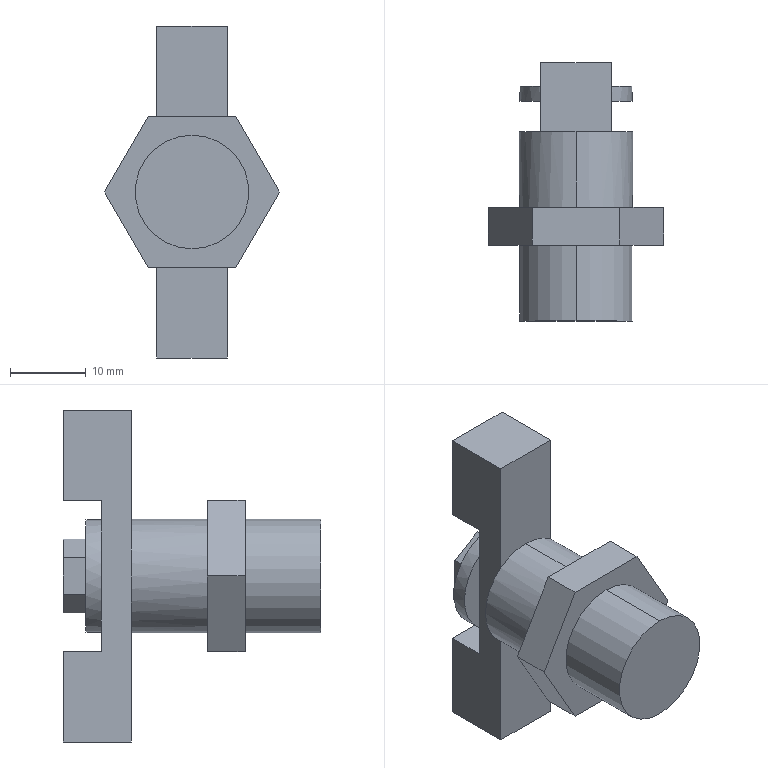Part | SolidWorks | features ICE 8, Extrusion 1 | 1 solid | 65 faces | box 23.094 x 34.03 x 43.8 mm | volume 8517 mm3 | plane 55 | cylinder 10 | commonest cylinder face diameters 5.701 x4 15 x4 14.848 x2